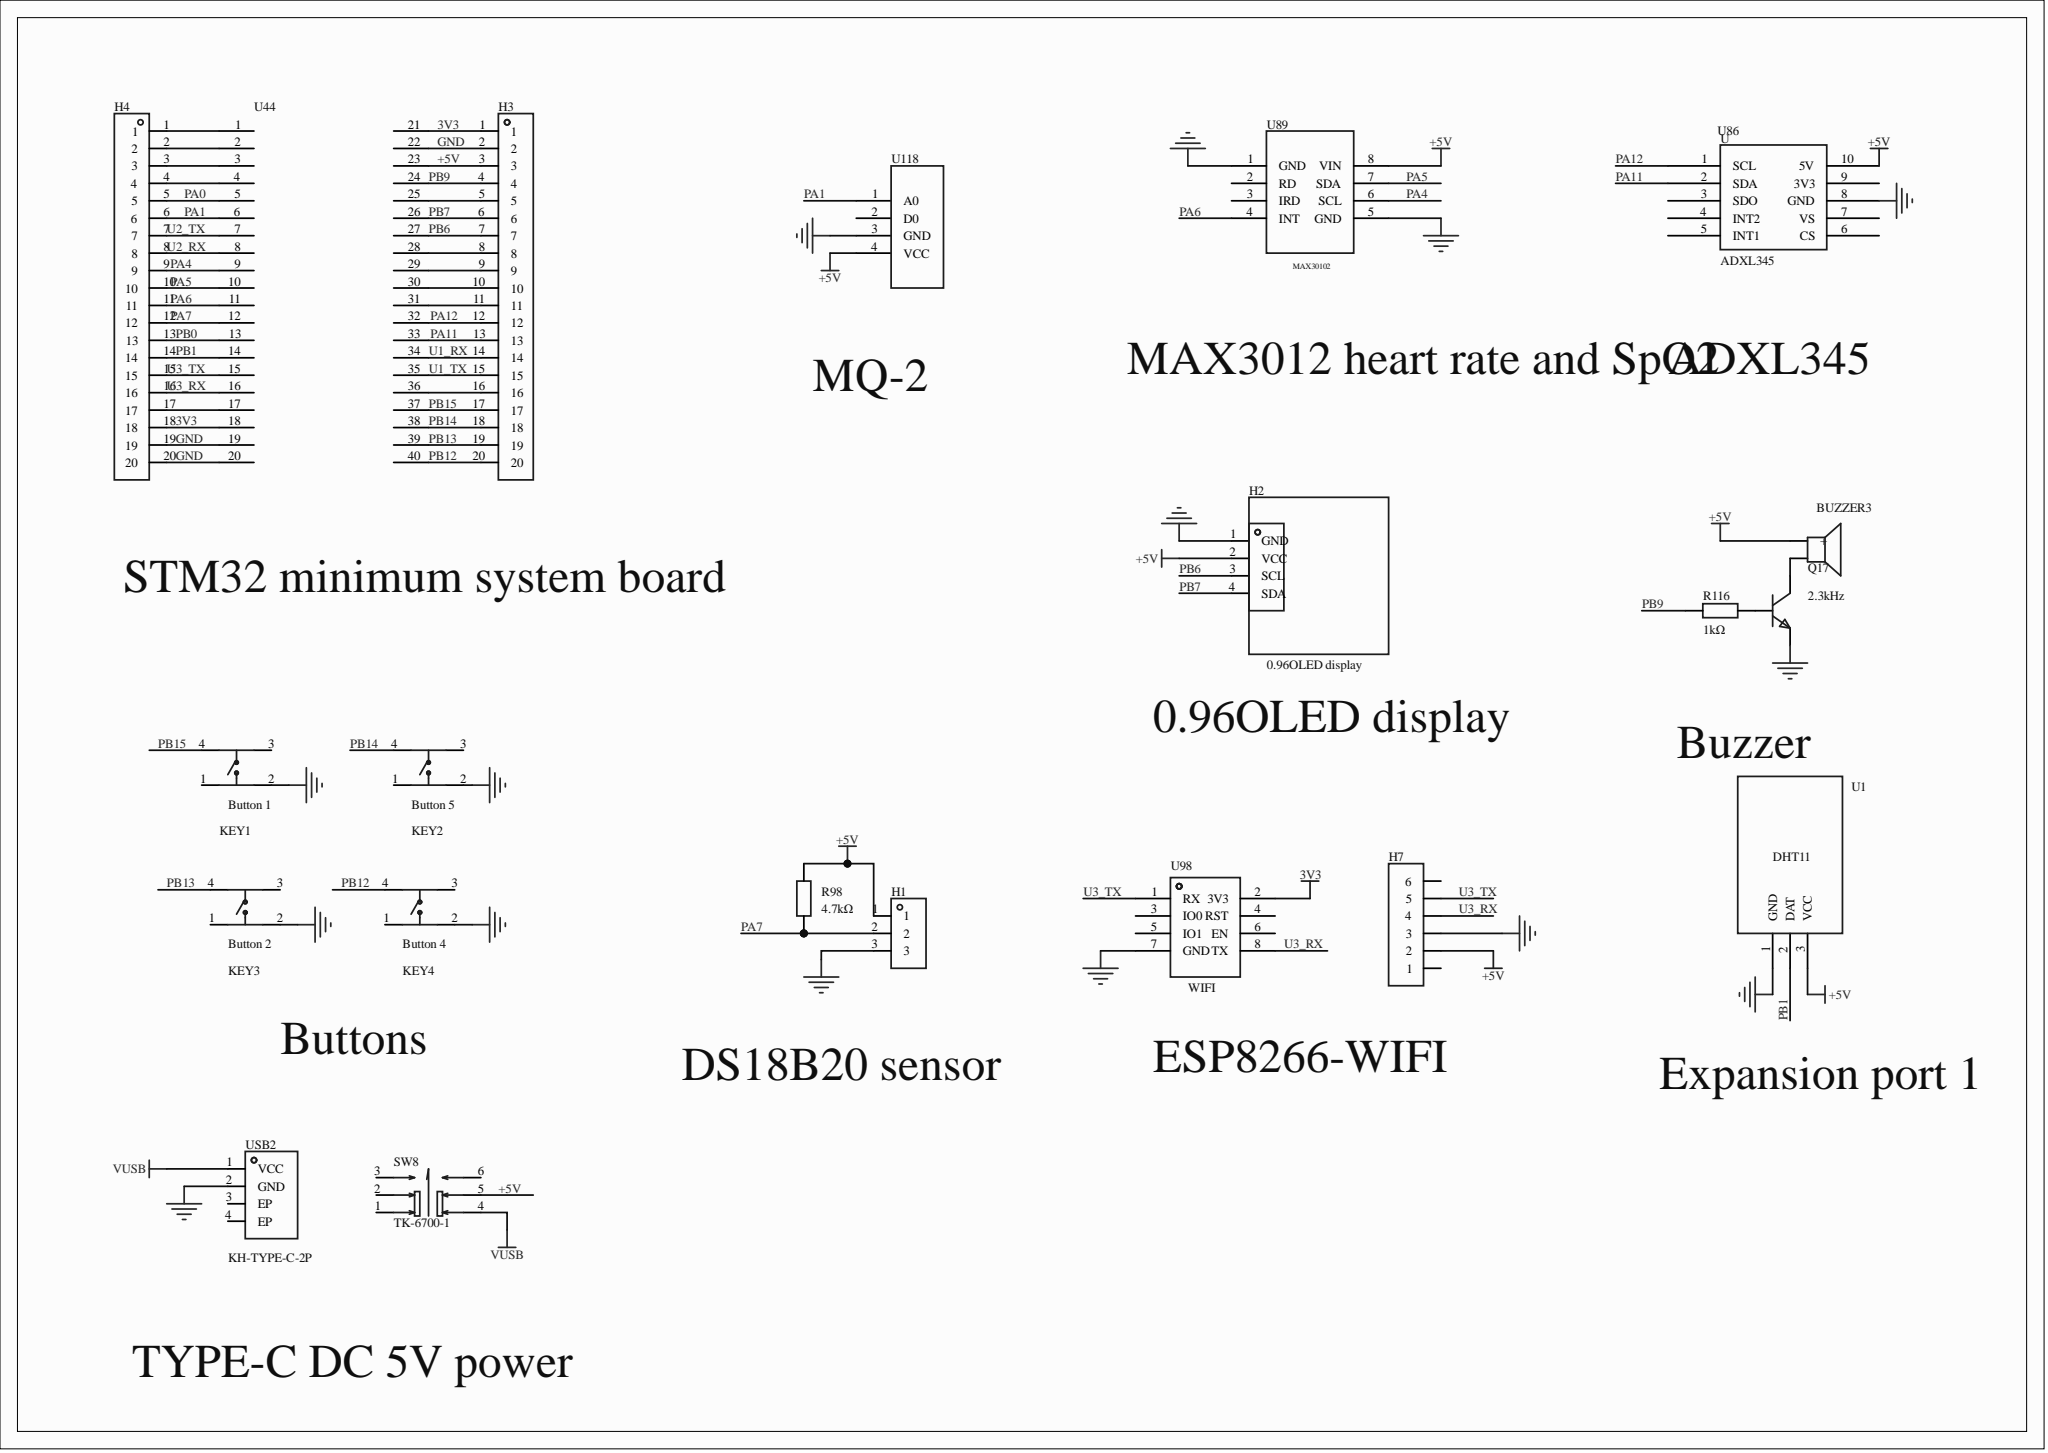Circuit board | Altium Designer | 21 parts | 40 nets
Bill of materials:
Comment,Description,Designator,Footprint,LibRef,Quantity
"2.3kHz","","BUZZER3","BUZ-TH_BD12.0-P7.60-D0.6-FD","TMB12A05_C96093","1"
"","","H1","HDR-TH_3P-P2.54-V-F","HDR-F_2.54_1x3P","1"
"2.54-1*4P female","","H2","HDR-TH_4P-P2.54-V-F","0.96OLED屏幕","1"
"","","H3, H4","HDR-TH_20P-P2.54-V-M-1","HDR-M_2.54_1x20P","2"
"","","H7","HDR-TH_6P-P2.54-V-M-1","HDR-M_2.54_1x6P","1"
"Button 1","","KEY1","KEY-TH_4P-L6.0-W6.0-P4.50-LS7.5","按键开关6*6*8","1"
"Button 5","","KEY2","KEY-TH_4P-L6.0-W6.0-P4.50-LS7.5","按键开关6*6*8","1"
"Button 2","","KEY3","KEY-TH_4P-L6.0-W6.0-P4.50-LS7.5","按键开关6*6*8","1"
"Button 4","","KEY4","KEY-TH_4P-L6.0-W6.0-P4.50-LS7.5","按键开关6*6*8","1"
"","","Q17","S8050_TO_92","S8050_TO_NPN","1"
"4.7kΩ","","R98","Res_1/4W","Res_AXIAL-1/4W","1"
"1kΩ","","R116","Res_1/4W","Res_AXIAL-1/4W","1"
"TK-6700-1","","SW8","SW-TH_TK-6700-1","TK-6700-1","1"
"","","U1","温湿度","温湿度DHT11","1"
"","","U44","STM32最小系统板","STM32最小系统板","1"
"","","U86","ADXL345","ADXL345","1"
"","","U89","MAX30102","MAX30102","1"
"","","U98","WiFi封装","WiFi模块","1"
"","","U118","MQ-X插件","MQ-X插件","1"
"KH-TYPE-C-2P","","USB2","USB-SMD_KH-TYPE-C-2P","KH-TYPE-C-2P","1"
Netlist (Protel format):
[
BUZZER3
BUZ-TH_BD12.0-P7.60-D0.6-FD
2.3kHz



]
[
H1
HDR-TH_3P-P2.54-V-F




]
[
H2
HDR-TH_4P-P2.54-V-F
2.54-1*4P female



]
[
H3
HDR-TH_20P-P2.54-V-M-1




]
[
H4
HDR-TH_20P-P2.54-V-M-1




]
[
H7
HDR-TH_6P-P2.54-V-M-1




]
[
KEY1
KEY-TH_4P-L6.0-W6.0-P4.50-LS7.5
Button 1



]
[
KEY2
KEY-TH_4P-L6.0-W6.0-P4.50-LS7.5
Button 5



]
[
KEY3
KEY-TH_4P-L6.0-W6.0-P4.50-LS7.5
Button 2



]
[
KEY4
KEY-TH_4P-L6.0-W6.0-P4.50-LS7.5
Button 4



]
[
Q17
S8050_TO_92




]
[
R98
Res_1/4W
4.7kΩ



]
[
R116
Res_1/4W
1kΩ



]
[
SW8
SW-TH_TK-6700-1
TK-6700-1



]
[
U1
温湿度




]
[
U44
STM32最小系统板




]
[
U86
ADXL345




]
[
U89
MAX30102




]
[
U98
WiFi封装




]
[
U118
MQ-X插件




]
[
USB2
USB-SMD_KH-TYPE-C-2P
KH-TYPE-C-2P



]
(
VUSB
SW8-4
USB2-1
)
(
U3_TX
H4-15
H7-5
U44-15
U98-1
)
(
U3_RX
H4-16
H7-4
U44-16
U98-8
)
(
U2_TX
H4-7
U44-7
)
(
U2_RX
H4-8
U44-8
)
(
U1_TX
H3-15
U44-35
)
(
U1_RX
H3-14
U44-34
)
(
PB15
H3-17
KEY1-4
U44-37
)
(
PB14
H3-18
KEY2-4
U44-38
)
(
PB13
H3-19
KEY3-4
U44-39
)
(
PB12
H3-20
KEY4-4
U44-40
)
(
PB9
H3-4
R116-1
U44-24
)
(
PB7
H2-4
H3-6
U44-26
)
(
PB6
H2-3
H3-7
U44-27
)
(
PB1
H4-14
U1-2
U44-14
)
(
PB0
H4-13
U44-13
)
(
PA12
H3-12
U44-32
U86-1
)
(
PA11
H3-13
U44-33
U86-2
)
(
PA7
H1-2
H4-12
R98-1
U44-12
)
(
PA6
H4-11
U44-11
U89-4
)
(
PA5
H4-10
U44-10
U89-7
)
(
PA4
H4-9
U44-9
U89-6
)
(
PA1
H4-6
U44-6
U118-1
)
(
PA0
H4-5
U44-5
)
(
NetQ17_2
Q17-2
R116-2
)
(
NetH4_17
H4-17
U44-17
)
(
NetH4_4
H4-4
U44-4
)
(
NetH4_3
H4-3
U44-3
)
(
NetH4_2
H4-2
U44-2
)
(
NetH4_1
H4-1
U44-1
)
(
NetH3_16
H3-16
U44-36
)
(
NetH3_11
H3-11
U44-31
)
(
NetH3_10
H3-10
U44-30
)
(
NetH3_9
H3-9
U44-29
)
(
NetH3_8
H3-8
U44-28
)
(
NetH3_5
H3-5
U44-25
)
(
NetBUZZER3_2
BUZZER3-2
Q17-3
)
(
GND
H1-3
H2-1
H3-2
H4-19
H4-20
H7-3
KEY1-2
KEY2-2
KEY3-2
KEY4-2
Q17-1
U1-1
U44-19
U44-20
U44-22
U86-8
U89-1
U89-5
U98-7
U118-3
USB2-2
)
(
+5V
BUZZER3-1
H1-1
H2-2
H3-3
H7-2
R98-2
SW8-5
U1-3
U44-23
U86-10
U89-8
U118-4
)
(
3V3
H3-1
H4-18
U44-18
U44-21
U98-2
)